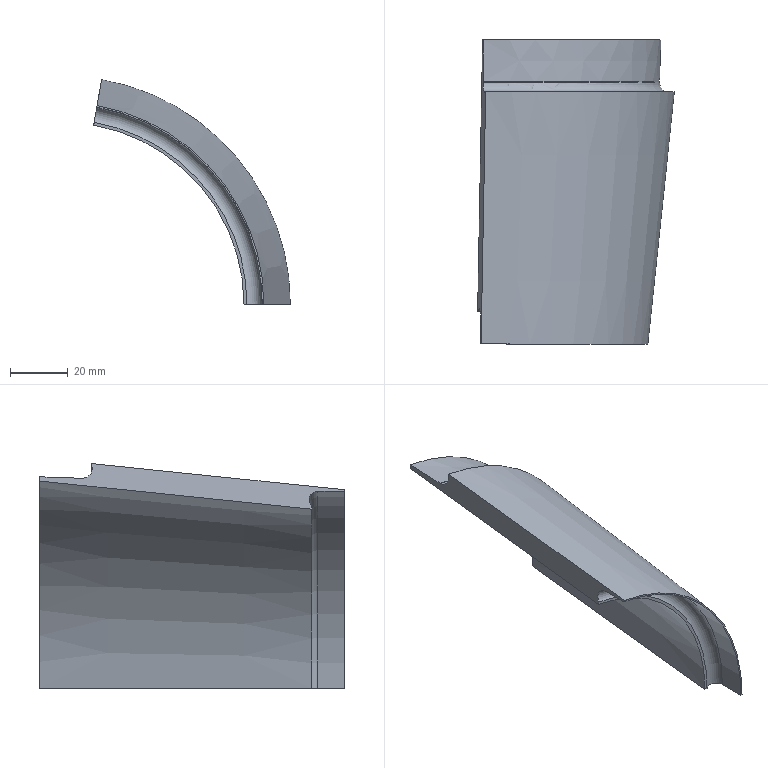Part | STEP file | rubber3 | 1 solid | 13 faces | box 68.197 x 105.496 x 77.952 mm | volume 66050 mm3 | plane 6 | cone 4 | torus 3
STEP:
#1=CARTESIAN_POINT('',(12.847,-92.752,72.857));
#2=VERTEX_POINT('',#1);
#3=CARTESIAN_POINT('',(12.847,-92.628,72.86));
#4=VERTEX_POINT('',#3);
#5=CARTESIAN_POINT('',(13.454,-92.752,76.302));
#6=DIRECTION('',(0.9848,0.,-0.1736));
#7=DIRECTION('',(0.1736,0.,0.9848));
#8=AXIS2_PLACEMENT_3D('',#5,#6,#7);
#9=CIRCLE('',#8,3.498);
#10=EDGE_CURVE('',#2,#4,#9,.T.);
#11=ORIENTED_EDGE('',*,*,#10,.F.);
#12=CARTESIAN_POINT('',(73.981,-92.752,0.));
#13=VERTEX_POINT('',#12);
#14=CARTESIAN_POINT('',(0.,-92.752,0.));
#15=DIRECTION('',(0.,1.,0.));
#16=DIRECTION('',(0.,0.,1.));
#17=AXIS2_PLACEMENT_3D('',#14,#15,#16);
#18=CIRCLE('',#17,73.981);
#19=EDGE_CURVE('',#2,#13,#18,.T.);
#20=ORIENTED_EDGE('',*,*,#19,.T.);
#21=CARTESIAN_POINT('',(73.983,-92.628,0.));
#22=VERTEX_POINT('',#21);
#23=CARTESIAN_POINT('',(77.479,-92.752,0.));
#24=DIRECTION('',(0.,0.,-1.));
#25=DIRECTION('',(1.,0.,0.));
#26=AXIS2_PLACEMENT_3D('',#23,#24,#25);
#27=CIRCLE('',#26,3.498);
#28=EDGE_CURVE('',#13,#22,#27,.T.);
#29=ORIENTED_EDGE('',*,*,#28,.T.);
#30=CARTESIAN_POINT('',(0.,-92.628,0.));
#31=DIRECTION('',(0.,1.,0.));
#32=DIRECTION('',(0.,0.,1.));
#33=AXIS2_PLACEMENT_3D('',#30,#31,#32);
#34=CIRCLE('',#33,73.983);
#35=EDGE_CURVE('',#4,#22,#34,.T.);
#36=ORIENTED_EDGE('',*,*,#35,.F.);
#37=EDGE_LOOP('',(#11,#20,#29,#36));
#38=FACE_OUTER_BOUND('',#37,.T.);
#39=CARTESIAN_POINT('',(0.,-92.752,0.));
#40=DIRECTION('',(0.,1.,0.));
#41=DIRECTION('',(0.,0.,1.));
#42=AXIS2_PLACEMENT_3D('',#39,#40,#41);
#43=TOROIDAL_SURFACE('',#42,77.479,3.498);
#44=ADVANCED_FACE('',(#38),#43,.F.);
#45=CARTESIAN_POINT('',(12.676,-78.068,71.891));
#46=VERTEX_POINT('',#45);
#47=CARTESIAN_POINT('',(73.,-78.068,0.));
#48=VERTEX_POINT('',#47);
#49=CARTESIAN_POINT('',(0.,-78.068,0.));
#50=DIRECTION('',(0.,1.,0.));
#51=DIRECTION('',(0.,0.,1.));
#52=AXIS2_PLACEMENT_3D('',#49,#50,#51);
#53=CIRCLE('',#52,73.);
#54=EDGE_CURVE('',#46,#48,#53,.T.);
#55=ORIENTED_EDGE('',*,*,#54,.F.);
#56=CARTESIAN_POINT('',(12.937,-78.068,73.368));
#57=VERTEX_POINT('',#56);
#58=CARTESIAN_POINT('',(12.676,-78.068,71.891));
#59=DIRECTION('',(-0.1736,0.,-0.9848));
#60=VECTOR('',#59,1000.);
#61=LINE('',#58,#60);
#62=EDGE_CURVE('',#57,#46,#61,.T.);
#63=ORIENTED_EDGE('',*,*,#62,.F.);
#64=CARTESIAN_POINT('',(74.5,-78.068,0.));
#65=VERTEX_POINT('',#64);
#66=CARTESIAN_POINT('',(0.,-78.068,0.));
#67=DIRECTION('',(0.,1.,0.));
#68=DIRECTION('',(0.,0.,1.));
#69=AXIS2_PLACEMENT_3D('',#66,#67,#68);
#70=CIRCLE('',#69,74.5);
#71=EDGE_CURVE('',#57,#65,#70,.T.);
#72=ORIENTED_EDGE('',*,*,#71,.T.);
#73=CARTESIAN_POINT('',(73.,-78.068,0.));
#74=DIRECTION('',(-1.,0.,0.));
#75=VECTOR('',#74,1000.);
#76=LINE('',#73,#75);
#77=EDGE_CURVE('',#65,#48,#76,.T.);
#78=ORIENTED_EDGE('',*,*,#77,.T.);
#79=EDGE_LOOP('',(#55,#63,#72,#78));
#80=FACE_OUTER_BOUND('',#79,.T.);
#81=CARTESIAN_POINT('',(12.676,-78.068,71.891));
#82=DIRECTION('',(0.,-1.,0.));
#83=DIRECTION('',(0.,0.,-1.));
#84=AXIS2_PLACEMENT_3D('',#81,#82,#83);
#85=PLANE('',#84);
#86=ADVANCED_FACE('',(#80),#85,.F.);
#87=CARTESIAN_POINT('',(10.957,-172.263,62.141));
#88=VERTEX_POINT('',#87);
#89=CARTESIAN_POINT('',(63.1,-172.263,0.));
#90=VERTEX_POINT('',#89);
#91=CARTESIAN_POINT('',(0.,-172.263,0.));
#92=DIRECTION('',(0.,1.,0.));
#93=DIRECTION('',(0.,0.,1.));
#94=AXIS2_PLACEMENT_3D('',#91,#92,#93);
#95=CIRCLE('',#94,63.1);
#96=EDGE_CURVE('',#88,#90,#95,.T.);
#97=ORIENTED_EDGE('',*,*,#96,.F.);
#98=CARTESIAN_POINT('',(12.676,-78.068,71.891));
#99=DIRECTION('',(-0.01815,-0.9945,-0.1029));
#100=VECTOR('',#99,1000.);
#101=LINE('',#98,#100);
#102=EDGE_CURVE('',#46,#88,#101,.T.);
#103=ORIENTED_EDGE('',*,*,#102,.F.);
#104=ORIENTED_EDGE('',*,*,#54,.T.);
#105=CARTESIAN_POINT('',(73.,-78.068,0.));
#106=DIRECTION('',(-0.1045,-0.9945,0.));
#107=VECTOR('',#106,1000.);
#108=LINE('',#105,#107);
#109=EDGE_CURVE('',#48,#90,#108,.T.);
#110=ORIENTED_EDGE('',*,*,#109,.T.);
#111=EDGE_LOOP('',(#97,#103,#104,#110));
#112=FACE_OUTER_BOUND('',#111,.T.);
#113=CARTESIAN_POINT('',(0.,-78.068,0.));
#114=DIRECTION('',(0.,1.,0.));
#115=DIRECTION('',(0.,0.,1.));
#116=AXIS2_PLACEMENT_3D('',#113,#114,#115);
#117=CONICAL_SURFACE('',#116,73.,0.1047);
#118=ADVANCED_FACE('',(#112),#117,.F.);
#119=CARTESIAN_POINT('',(11.131,-172.263,63.126));
#120=VERTEX_POINT('',#119);
#121=CARTESIAN_POINT('',(64.1,-172.263,0.));
#122=VERTEX_POINT('',#121);
#123=CARTESIAN_POINT('',(0.,-172.263,0.));
#124=DIRECTION('',(0.,1.,0.));
#125=DIRECTION('',(0.,0.,1.));
#126=AXIS2_PLACEMENT_3D('',#123,#124,#125);
#127=CIRCLE('',#126,64.1);
#128=EDGE_CURVE('',#120,#122,#127,.T.);
#129=ORIENTED_EDGE('',*,*,#128,.F.);
#130=CARTESIAN_POINT('',(10.957,-172.263,62.141));
#131=DIRECTION('',(0.1736,0.,0.9848));
#132=VECTOR('',#131,1000.);
#133=LINE('',#130,#132);
#134=EDGE_CURVE('',#88,#120,#133,.T.);
#135=ORIENTED_EDGE('',*,*,#134,.F.);
#136=ORIENTED_EDGE('',*,*,#96,.T.);
#137=CARTESIAN_POINT('',(63.1,-172.263,0.));
#138=DIRECTION('',(1.,0.,0.));
#139=VECTOR('',#138,1000.);
#140=LINE('',#137,#139);
#141=EDGE_CURVE('',#90,#122,#140,.T.);
#142=ORIENTED_EDGE('',*,*,#141,.T.);
#143=EDGE_LOOP('',(#129,#135,#136,#142));
#144=FACE_OUTER_BOUND('',#143,.T.);
#145=CARTESIAN_POINT('',(10.957,-172.263,62.141));
#146=DIRECTION('',(0.,1.,0.));
#147=DIRECTION('',(0.,0.,1.));
#148=AXIS2_PLACEMENT_3D('',#145,#146,#147);
#149=PLANE('',#148);
#150=ADVANCED_FACE('',(#144),#149,.F.);
#151=CARTESIAN_POINT('',(12.052,-174.481,68.348));
#152=VERTEX_POINT('',#151);
#153=CARTESIAN_POINT('',(69.402,-174.481,0.));
#154=VERTEX_POINT('',#153);
#155=CARTESIAN_POINT('',(0.,-174.481,0.));
#156=DIRECTION('',(0.,1.,0.));
#157=DIRECTION('',(0.,0.,1.));
#158=AXIS2_PLACEMENT_3D('',#155,#156,#157);
#159=CIRCLE('',#158,69.402);
#160=EDGE_CURVE('',#152,#154,#159,.T.);
#161=ORIENTED_EDGE('',*,*,#160,.F.);
#162=CARTESIAN_POINT('',(11.509,-174.5,65.272));
#163=DIRECTION('',(0.9848,0.,-0.1736));
#164=DIRECTION('',(0.1736,0.,0.9848));
#165=AXIS2_PLACEMENT_3D('',#162,#163,#164);
#166=CIRCLE('',#165,3.123);
#167=EDGE_CURVE('',#120,#152,#166,.T.);
#168=ORIENTED_EDGE('',*,*,#167,.F.);
#169=ORIENTED_EDGE('',*,*,#128,.T.);
#170=CARTESIAN_POINT('',(66.279,-174.5,0.));
#171=DIRECTION('',(0.,0.,-1.));
#172=DIRECTION('',(1.,0.,0.));
#173=AXIS2_PLACEMENT_3D('',#170,#171,#172);
#174=CIRCLE('',#173,3.123);
#175=EDGE_CURVE('',#122,#154,#174,.T.);
#176=ORIENTED_EDGE('',*,*,#175,.T.);
#177=EDGE_LOOP('',(#161,#168,#169,#176));
#178=FACE_OUTER_BOUND('',#177,.T.);
#179=CARTESIAN_POINT('',(0.,-174.5,0.));
#180=DIRECTION('',(0.,1.,0.));
#181=DIRECTION('',(0.,0.,1.));
#182=AXIS2_PLACEMENT_3D('',#179,#180,#181);
#183=TOROIDAL_SURFACE('',#182,66.279,3.123);
#184=ADVANCED_FACE('',(#178),#183,.F.);
#185=CARTESIAN_POINT('',(12.061,-183.564,68.401));
#186=VERTEX_POINT('',#185);
#187=CARTESIAN_POINT('',(69.456,-183.564,0.));
#188=VERTEX_POINT('',#187);
#189=CARTESIAN_POINT('',(0.,-183.564,0.));
#190=DIRECTION('',(0.,1.,0.));
#191=DIRECTION('',(0.,0.,1.));
#192=AXIS2_PLACEMENT_3D('',#189,#190,#191);
#193=CIRCLE('',#192,69.456);
#194=EDGE_CURVE('',#186,#188,#193,.T.);
#195=ORIENTED_EDGE('',*,*,#194,.F.);
#196=CARTESIAN_POINT('',(12.052,-174.481,68.348));
#197=DIRECTION('',(0.001025,-1.,0.005811));
#198=VECTOR('',#197,1000.);
#199=LINE('',#196,#198);
#200=EDGE_CURVE('',#152,#186,#199,.T.);
#201=ORIENTED_EDGE('',*,*,#200,.F.);
#202=ORIENTED_EDGE('',*,*,#160,.T.);
#203=CARTESIAN_POINT('',(69.402,-174.481,0.));
#204=DIRECTION('',(0.005901,-1.,0.));
#205=VECTOR('',#204,1000.);
#206=LINE('',#203,#205);
#207=EDGE_CURVE('',#154,#188,#206,.T.);
#208=ORIENTED_EDGE('',*,*,#207,.T.);
#209=EDGE_LOOP('',(#195,#201,#202,#208));
#210=FACE_OUTER_BOUND('',#209,.T.);
#211=CARTESIAN_POINT('',(0.,-174.481,0.));
#212=DIRECTION('',(0.,-1.,0.));
#213=DIRECTION('',(0.,0.,-1.));
#214=AXIS2_PLACEMENT_3D('',#211,#212,#213);
#215=CONICAL_SURFACE('',#214,69.402,0.005901);
#216=ADVANCED_FACE('',(#210),#215,.F.);
#217=CARTESIAN_POINT('',(12.148,-183.564,68.893));
#218=VERTEX_POINT('',#217);
#219=CARTESIAN_POINT('',(69.956,-183.564,0.));
#220=VERTEX_POINT('',#219);
#221=CARTESIAN_POINT('',(0.,-183.564,0.));
#222=DIRECTION('',(0.,1.,0.));
#223=DIRECTION('',(0.,0.,1.));
#224=AXIS2_PLACEMENT_3D('',#221,#222,#223);
#225=CIRCLE('',#224,69.956);
#226=EDGE_CURVE('',#218,#220,#225,.T.);
#227=ORIENTED_EDGE('',*,*,#226,.F.);
#228=CARTESIAN_POINT('',(12.148,-183.564,68.893));
#229=DIRECTION('',(0.1736,0.,0.9848));
#230=VECTOR('',#229,1000.);
#231=LINE('',#228,#230);
#232=EDGE_CURVE('',#186,#218,#231,.T.);
#233=ORIENTED_EDGE('',*,*,#232,.F.);
#234=ORIENTED_EDGE('',*,*,#194,.T.);
#235=CARTESIAN_POINT('',(69.956,-183.564,0.));
#236=DIRECTION('',(1.,0.,0.));
#237=VECTOR('',#236,1000.);
#238=LINE('',#235,#237);
#239=EDGE_CURVE('',#188,#220,#238,.T.);
#240=ORIENTED_EDGE('',*,*,#239,.T.);
#241=EDGE_LOOP('',(#227,#233,#234,#240));
#242=FACE_OUTER_BOUND('',#241,.T.);
#243=CARTESIAN_POINT('',(12.148,-183.564,68.893));
#244=DIRECTION('',(0.,1.,0.));
#245=DIRECTION('',(0.,0.,1.));
#246=AXIS2_PLACEMENT_3D('',#243,#244,#245);
#247=PLANE('',#246);
#248=ADVANCED_FACE('',(#242),#247,.F.);
#249=CARTESIAN_POINT('',(13.745,-96.046,77.952));
#250=VERTEX_POINT('',#249);
#251=CARTESIAN_POINT('',(79.154,-96.046,0.));
#252=VERTEX_POINT('',#251);
#253=CARTESIAN_POINT('',(0.,-96.046,0.));
#254=DIRECTION('',(0.,1.,0.));
#255=DIRECTION('',(0.,0.,1.));
#256=AXIS2_PLACEMENT_3D('',#253,#254,#255);
#257=CIRCLE('',#256,79.154);
#258=EDGE_CURVE('',#250,#252,#257,.T.);
#259=ORIENTED_EDGE('',*,*,#258,.F.);
#260=CARTESIAN_POINT('',(13.745,-96.046,77.952));
#261=DIRECTION('',(0.01815,0.9945,0.1029));
#262=VECTOR('',#261,1000.);
#263=LINE('',#260,#262);
#264=EDGE_CURVE('',#218,#250,#263,.T.);
#265=ORIENTED_EDGE('',*,*,#264,.F.);
#266=ORIENTED_EDGE('',*,*,#226,.T.);
#267=CARTESIAN_POINT('',(79.154,-96.046,0.));
#268=DIRECTION('',(0.1045,0.9945,0.));
#269=VECTOR('',#268,1000.);
#270=LINE('',#267,#269);
#271=EDGE_CURVE('',#220,#252,#270,.T.);
#272=ORIENTED_EDGE('',*,*,#271,.T.);
#273=EDGE_LOOP('',(#259,#265,#266,#272));
#274=FACE_OUTER_BOUND('',#273,.T.);
#275=CARTESIAN_POINT('',(0.,-183.564,0.));
#276=DIRECTION('',(0.,1.,0.));
#277=DIRECTION('',(0.,0.,1.));
#278=AXIS2_PLACEMENT_3D('',#275,#276,#277);
#279=CONICAL_SURFACE('',#278,69.956,0.1047);
#280=ADVANCED_FACE('',(#274),#279,.T.);
#281=CARTESIAN_POINT('',(13.658,-96.046,77.46));
#282=VERTEX_POINT('',#281);
#283=CARTESIAN_POINT('',(78.654,-96.046,0.));
#284=VERTEX_POINT('',#283);
#285=CARTESIAN_POINT('',(0.,-96.046,0.));
#286=DIRECTION('',(0.,1.,0.));
#287=DIRECTION('',(0.,0.,1.));
#288=AXIS2_PLACEMENT_3D('',#285,#286,#287);
#289=CIRCLE('',#288,78.654);
#290=EDGE_CURVE('',#282,#284,#289,.T.);
#291=ORIENTED_EDGE('',*,*,#290,.F.);
#292=CARTESIAN_POINT('',(13.745,-96.046,77.952));
#293=DIRECTION('',(-0.1736,0.,-0.9848));
#294=VECTOR('',#293,1000.);
#295=LINE('',#292,#294);
#296=EDGE_CURVE('',#250,#282,#295,.T.);
#297=ORIENTED_EDGE('',*,*,#296,.F.);
#298=ORIENTED_EDGE('',*,*,#258,.T.);
#299=CARTESIAN_POINT('',(79.154,-96.046,0.));
#300=DIRECTION('',(-1.,0.,0.));
#301=VECTOR('',#300,1000.);
#302=LINE('',#299,#301);
#303=EDGE_CURVE('',#252,#284,#302,.T.);
#304=ORIENTED_EDGE('',*,*,#303,.T.);
#305=EDGE_LOOP('',(#291,#297,#298,#304));
#306=FACE_OUTER_BOUND('',#305,.T.);
#307=CARTESIAN_POINT('',(13.745,-96.046,77.952));
#308=DIRECTION('',(0.,-1.,0.));
#309=DIRECTION('',(0.,0.,-1.));
#310=AXIS2_PLACEMENT_3D('',#307,#308,#309);
#311=PLANE('',#310);
#312=ADVANCED_FACE('',(#306),#311,.F.);
#313=ORIENTED_EDGE('',*,*,#19,.F.);
#314=CARTESIAN_POINT('',(13.454,-92.752,76.302));
#315=DIRECTION('',(0.9848,0.,-0.1736));
#316=DIRECTION('',(0.1736,0.,0.9848));
#317=AXIS2_PLACEMENT_3D('',#314,#315,#316);
#318=CIRCLE('',#317,3.498);
#319=EDGE_CURVE('',#282,#2,#318,.T.);
#320=ORIENTED_EDGE('',*,*,#319,.F.);
#321=ORIENTED_EDGE('',*,*,#290,.T.);
#322=CARTESIAN_POINT('',(77.479,-92.752,0.));
#323=DIRECTION('',(0.,0.,-1.));
#324=DIRECTION('',(1.,0.,0.));
#325=AXIS2_PLACEMENT_3D('',#322,#323,#324);
#326=CIRCLE('',#325,3.498);
#327=EDGE_CURVE('',#284,#13,#326,.T.);
#328=ORIENTED_EDGE('',*,*,#327,.T.);
#329=EDGE_LOOP('',(#313,#320,#321,#328));
#330=FACE_OUTER_BOUND('',#329,.T.);
#331=CARTESIAN_POINT('',(0.,-92.752,0.));
#332=DIRECTION('',(0.,1.,0.));
#333=DIRECTION('',(0.,0.,1.));
#334=AXIS2_PLACEMENT_3D('',#331,#332,#333);
#335=TOROIDAL_SURFACE('',#334,77.479,3.498);
#336=ADVANCED_FACE('',(#330),#335,.F.);
#337=CARTESIAN_POINT('',(12.937,-78.068,73.368));
#338=DIRECTION('',(0.006156,0.9994,0.03491));
#339=VECTOR('',#338,1000.);
#340=LINE('',#337,#339);
#341=EDGE_CURVE('',#4,#57,#340,.T.);
#342=ORIENTED_EDGE('',*,*,#341,.F.);
#343=ORIENTED_EDGE('',*,*,#35,.T.);
#344=CARTESIAN_POINT('',(74.5,-78.068,0.));
#345=DIRECTION('',(0.03545,0.9994,0.));
#346=VECTOR('',#345,1000.);
#347=LINE('',#344,#346);
#348=EDGE_CURVE('',#22,#65,#347,.T.);
#349=ORIENTED_EDGE('',*,*,#348,.T.);
#350=ORIENTED_EDGE('',*,*,#71,.F.);
#351=EDGE_LOOP('',(#342,#343,#349,#350));
#352=FACE_OUTER_BOUND('',#351,.T.);
#353=CARTESIAN_POINT('',(0.,-92.628,0.));
#354=DIRECTION('',(0.,1.,0.));
#355=DIRECTION('',(0.,0.,1.));
#356=AXIS2_PLACEMENT_3D('',#353,#354,#355);
#357=CONICAL_SURFACE('',#356,73.983,0.03546);
#358=ADVANCED_FACE('',(#352),#357,.T.);
#359=ORIENTED_EDGE('',*,*,#62,.T.);
#360=ORIENTED_EDGE('',*,*,#102,.T.);
#361=ORIENTED_EDGE('',*,*,#134,.T.);
#362=ORIENTED_EDGE('',*,*,#167,.T.);
#363=ORIENTED_EDGE('',*,*,#200,.T.);
#364=ORIENTED_EDGE('',*,*,#232,.T.);
#365=ORIENTED_EDGE('',*,*,#264,.T.);
#366=ORIENTED_EDGE('',*,*,#296,.T.);
#367=ORIENTED_EDGE('',*,*,#319,.T.);
#368=ORIENTED_EDGE('',*,*,#10,.T.);
#369=ORIENTED_EDGE('',*,*,#341,.T.);
#370=EDGE_LOOP('',(#359,#360,#361,#362,#363,#364,#365,#366,#367,#368,#369));
#371=FACE_OUTER_BOUND('',#370,.T.);
#372=CARTESIAN_POINT('',(13.454,-92.752,76.302));
#373=DIRECTION('',(-0.9848,0.,0.1736));
#374=DIRECTION('',(0.1736,0.,0.9848));
#375=AXIS2_PLACEMENT_3D('',#372,#373,#374);
#376=PLANE('',#375);
#377=ADVANCED_FACE('',(#371),#376,.T.);
#378=ORIENTED_EDGE('',*,*,#77,.F.);
#379=ORIENTED_EDGE('',*,*,#348,.F.);
#380=ORIENTED_EDGE('',*,*,#28,.F.);
#381=ORIENTED_EDGE('',*,*,#327,.F.);
#382=ORIENTED_EDGE('',*,*,#303,.F.);
#383=ORIENTED_EDGE('',*,*,#271,.F.);
#384=ORIENTED_EDGE('',*,*,#239,.F.);
#385=ORIENTED_EDGE('',*,*,#207,.F.);
#386=ORIENTED_EDGE('',*,*,#175,.F.);
#387=ORIENTED_EDGE('',*,*,#141,.F.);
#388=ORIENTED_EDGE('',*,*,#109,.F.);
#389=EDGE_LOOP('',(#378,#379,#380,#381,#382,#383,#384,#385,#386,#387,#388));
#390=FACE_OUTER_BOUND('',#389,.T.);
#391=CARTESIAN_POINT('',(77.479,-92.752,0.));
#392=DIRECTION('',(0.,0.,1.));
#393=DIRECTION('',(1.,0.,0.));
#394=AXIS2_PLACEMENT_3D('',#391,#392,#393);
#395=PLANE('',#394);
#396=ADVANCED_FACE('',(#390),#395,.F.);
#397=CLOSED_SHELL('',(#44,#86,#118,#150,#184,#216,#248,#280,#312,#336,#358,#377,#396));
#398=MANIFOLD_SOLID_BREP('',#397);
#399=CARTESIAN_POINT('',(0.,0.,0.));
#400=DIRECTION('',(0.,0.,1.));
#401=DIRECTION('',(1.,0.,0.));
#402=AXIS2_PLACEMENT_3D('',#399,#400,#401);
#403=(LENGTH_UNIT()NAMED_UNIT(*)SI_UNIT(.MILLI.,.METRE.));
#404=UNCERTAINTY_MEASURE_WITH_UNIT(LENGTH_MEASURE(0.00001),#403,'','');
#405=(NAMED_UNIT(*)PLANE_ANGLE_UNIT()SI_UNIT($,.RADIAN.));
#406=(NAMED_UNIT(*)SI_UNIT($,.STERADIAN.)SOLID_ANGLE_UNIT());
#407=(GEOMETRIC_REPRESENTATION_CONTEXT(3)GLOBAL_UNCERTAINTY_ASSIGNED_CONTEXT((#404))GLOBAL_UNIT_ASSIGNED_CONTEXT((#403,#405,#406))REPRESENTATION_CONTEXT('',''));
#408=ADVANCED_BREP_SHAPE_REPRESENTATION('',(#398,#402),#407);